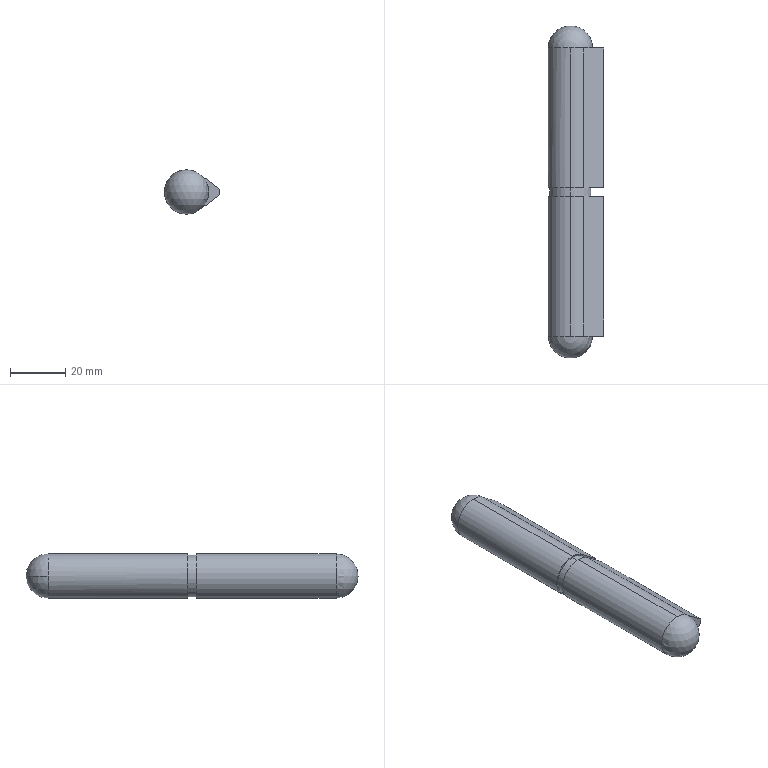Part | STEP file | GN 128.2-120-A41201611203204 | 2 solids | 30 faces | box 20 x 120 x 16 mm | volume 25167 mm3 | cylinder 12 | plane 11 | sphere 5 | cone 2 | commonest cylinder face diameters 16 x6 11 x4 15 x2